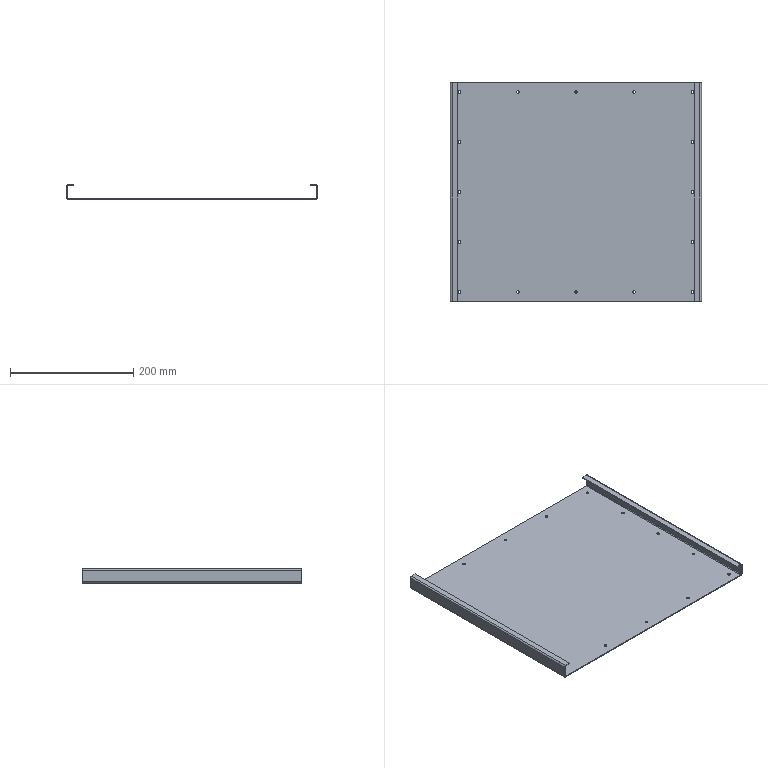Part | STEP file | Electrical box base plate | 1 solid | 54 faces | box 408 x 355 x 23 mm | volume 248875 mm3 | plane 30 | cylinder 24 | commonest cylinder face diameters 4.2 x16 2 x4 5 x4
STEP:
#1=CARTESIAN_POINT('',(10.,355.,-1.));
#2=VERTEX_POINT('',#1);
#3=CARTESIAN_POINT('',(11.5,355.,-1.));
#4=VERTEX_POINT('',#3);
#5=CARTESIAN_POINT('',(10.,355.,-1.));
#6=DIRECTION('',(1.,0.,0.));
#7=VECTOR('',#6,1000.);
#8=LINE('',#5,#7);
#9=EDGE_CURVE('',#2,#4,#8,.T.);
#10=ORIENTED_EDGE('',*,*,#9,.F.);
#11=CARTESIAN_POINT('',(9.,355.,0.));
#12=VERTEX_POINT('',#11);
#13=CARTESIAN_POINT('',(9.,355.,-1.));
#14=DIRECTION('',(0.,1.,0.));
#15=DIRECTION('',(0.,0.,-1.));
#16=AXIS2_PLACEMENT_3D('',#13,#14,#15);
#17=CIRCLE('',#16,1.);
#18=EDGE_CURVE('',#12,#2,#17,.T.);
#19=ORIENTED_EDGE('',*,*,#18,.F.);
#20=CARTESIAN_POINT('',(9.,355.,1.5));
#21=VERTEX_POINT('',#20);
#22=CARTESIAN_POINT('',(9.,355.,1.5));
#23=DIRECTION('',(0.,0.,-1.));
#24=VECTOR('',#23,1000.);
#25=LINE('',#22,#24);
#26=EDGE_CURVE('',#21,#12,#25,.T.);
#27=ORIENTED_EDGE('',*,*,#26,.F.);
#28=CARTESIAN_POINT('',(9.,355.,-1.));
#29=DIRECTION('',(0.,1.,0.));
#30=DIRECTION('',(1.,0.,0.));
#31=AXIS2_PLACEMENT_3D('',#28,#29,#30);
#32=CIRCLE('',#31,2.5);
#33=EDGE_CURVE('',#21,#4,#32,.T.);
#34=ORIENTED_EDGE('',*,*,#33,.T.);
#35=EDGE_LOOP('',(#10,#19,#27,#34));
#36=FACE_OUTER_BOUND('',#35,.T.);
#37=CARTESIAN_POINT('',(10.,355.,-1.));
#38=DIRECTION('',(0.,1.,0.));
#39=DIRECTION('',(0.,0.,1.));
#40=AXIS2_PLACEMENT_3D('',#37,#38,#39);
#41=PLANE('',#40);
#42=ADVANCED_FACE('',(#36),#41,.T.);
#43=CARTESIAN_POINT('',(10.,355.,-19.));
#44=VERTEX_POINT('',#43);
#45=CARTESIAN_POINT('',(10.,355.,0.));
#46=DIRECTION('',(0.,0.,-1.));
#47=VECTOR('',#46,1000.);
#48=LINE('',#45,#47);
#49=EDGE_CURVE('',#2,#44,#48,.T.);
#50=ORIENTED_EDGE('',*,*,#49,.F.);
#51=ORIENTED_EDGE('',*,*,#9,.T.);
#52=CARTESIAN_POINT('',(11.5,355.,-19.));
#53=VERTEX_POINT('',#52);
#54=CARTESIAN_POINT('',(11.5,355.,0.));
#55=DIRECTION('',(0.,0.,-1.));
#56=VECTOR('',#55,1000.);
#57=LINE('',#54,#56);
#58=EDGE_CURVE('',#4,#53,#57,.T.);
#59=ORIENTED_EDGE('',*,*,#58,.T.);
#60=CARTESIAN_POINT('',(11.5,355.,-19.));
#61=DIRECTION('',(-1.,0.,0.));
#62=VECTOR('',#61,1000.);
#63=LINE('',#60,#62);
#64=EDGE_CURVE('',#53,#44,#63,.T.);
#65=ORIENTED_EDGE('',*,*,#64,.T.);
#66=EDGE_LOOP('',(#50,#51,#59,#65));
#67=FACE_OUTER_BOUND('',#66,.T.);
#68=CARTESIAN_POINT('',(9.,355.,1.5));
#69=DIRECTION('',(0.,1.,0.));
#70=DIRECTION('',(0.,0.,1.));
#71=AXIS2_PLACEMENT_3D('',#68,#69,#70);
#72=PLANE('',#71);
#73=ADVANCED_FACE('',(#67),#72,.T.);
#74=CARTESIAN_POINT('',(9.,0.,0.));
#75=VERTEX_POINT('',#74);
#76=CARTESIAN_POINT('',(9.,0.,1.5));
#77=VERTEX_POINT('',#76);
#78=CARTESIAN_POINT('',(9.,0.,0.));
#79=DIRECTION('',(0.,0.,1.));
#80=VECTOR('',#79,1000.);
#81=LINE('',#78,#80);
#82=EDGE_CURVE('',#75,#77,#81,.T.);
#83=ORIENTED_EDGE('',*,*,#82,.F.);
#84=CARTESIAN_POINT('',(10.,0.,-1.));
#85=VERTEX_POINT('',#84);
#86=CARTESIAN_POINT('',(9.,0.,-1.));
#87=DIRECTION('',(0.,1.,0.));
#88=DIRECTION('',(0.,0.,-1.));
#89=AXIS2_PLACEMENT_3D('',#86,#87,#88);
#90=CIRCLE('',#89,1.);
#91=EDGE_CURVE('',#75,#85,#90,.T.);
#92=ORIENTED_EDGE('',*,*,#91,.T.);
#93=CARTESIAN_POINT('',(11.5,0.,-1.));
#94=VERTEX_POINT('',#93);
#95=CARTESIAN_POINT('',(11.5,0.,-1.));
#96=DIRECTION('',(-1.,0.,0.));
#97=VECTOR('',#96,1000.);
#98=LINE('',#95,#97);
#99=EDGE_CURVE('',#94,#85,#98,.T.);
#100=ORIENTED_EDGE('',*,*,#99,.F.);
#101=CARTESIAN_POINT('',(9.,0.,-1.));
#102=DIRECTION('',(0.,1.,0.));
#103=DIRECTION('',(1.,0.,0.));
#104=AXIS2_PLACEMENT_3D('',#101,#102,#103);
#105=CIRCLE('',#104,2.5);
#106=EDGE_CURVE('',#77,#94,#105,.T.);
#107=ORIENTED_EDGE('',*,*,#106,.F.);
#108=EDGE_LOOP('',(#83,#92,#100,#107));
#109=FACE_OUTER_BOUND('',#108,.T.);
#110=CARTESIAN_POINT('',(9.,0.,0.));
#111=DIRECTION('',(0.,-1.,0.));
#112=DIRECTION('',(0.,0.,-1.));
#113=AXIS2_PLACEMENT_3D('',#110,#111,#112);
#114=PLANE('',#113);
#115=ADVANCED_FACE('',(#109),#114,.T.);
#116=CARTESIAN_POINT('',(0.,0.,0.));
#117=VERTEX_POINT('',#116);
#118=CARTESIAN_POINT('',(0.,0.,0.));
#119=DIRECTION('',(1.,0.,0.));
#120=VECTOR('',#119,1000.);
#121=LINE('',#118,#120);
#122=EDGE_CURVE('',#117,#75,#121,.T.);
#123=ORIENTED_EDGE('',*,*,#122,.T.);
#124=ORIENTED_EDGE('',*,*,#82,.T.);
#125=CARTESIAN_POINT('',(0.,0.,1.5));
#126=VERTEX_POINT('',#125);
#127=CARTESIAN_POINT('',(0.,0.,1.5));
#128=DIRECTION('',(1.,0.,0.));
#129=VECTOR('',#128,1000.);
#130=LINE('',#127,#129);
#131=EDGE_CURVE('',#126,#77,#130,.T.);
#132=ORIENTED_EDGE('',*,*,#131,.F.);
#133=CARTESIAN_POINT('',(0.,0.,1.5));
#134=DIRECTION('',(0.,0.,-1.));
#135=VECTOR('',#134,1000.);
#136=LINE('',#133,#135);
#137=EDGE_CURVE('',#126,#117,#136,.T.);
#138=ORIENTED_EDGE('',*,*,#137,.T.);
#139=EDGE_LOOP('',(#123,#124,#132,#138));
#140=FACE_OUTER_BOUND('',#139,.T.);
#141=CARTESIAN_POINT('',(11.5,0.,-1.));
#142=DIRECTION('',(0.,-1.,0.));
#143=DIRECTION('',(0.,0.,-1.));
#144=AXIS2_PLACEMENT_3D('',#141,#142,#143);
#145=PLANE('',#144);
#146=ADVANCED_FACE('',(#140),#145,.T.);
#147=CARTESIAN_POINT('',(9.,355.,-20.));
#148=VERTEX_POINT('',#147);
#149=CARTESIAN_POINT('',(9.,355.,-21.5));
#150=VERTEX_POINT('',#149);
#151=CARTESIAN_POINT('',(9.,355.,-20.));
#152=DIRECTION('',(0.,0.,-1.));
#153=VECTOR('',#152,1000.);
#154=LINE('',#151,#153);
#155=EDGE_CURVE('',#148,#150,#154,.T.);
#156=ORIENTED_EDGE('',*,*,#155,.F.);
#157=CARTESIAN_POINT('',(9.,355.,-19.));
#158=DIRECTION('',(0.,1.,0.));
#159=DIRECTION('',(0.,0.,-1.));
#160=AXIS2_PLACEMENT_3D('',#157,#158,#159);
#161=CIRCLE('',#160,1.);
#162=EDGE_CURVE('',#44,#148,#161,.T.);
#163=ORIENTED_EDGE('',*,*,#162,.F.);
#164=ORIENTED_EDGE('',*,*,#64,.F.);
#165=CARTESIAN_POINT('',(9.,355.,-19.));
#166=DIRECTION('',(0.,1.,0.));
#167=DIRECTION('',(1.,0.,0.));
#168=AXIS2_PLACEMENT_3D('',#165,#166,#167);
#169=CIRCLE('',#168,2.5);
#170=EDGE_CURVE('',#53,#150,#169,.T.);
#171=ORIENTED_EDGE('',*,*,#170,.T.);
#172=EDGE_LOOP('',(#156,#163,#164,#171));
#173=FACE_OUTER_BOUND('',#172,.T.);
#174=CARTESIAN_POINT('',(9.,355.,-20.));
#175=DIRECTION('',(0.,1.,0.));
#176=DIRECTION('',(0.,0.,1.));
#177=AXIS2_PLACEMENT_3D('',#174,#175,#176);
#178=PLANE('',#177);
#179=ADVANCED_FACE('',(#173),#178,.T.);
#180=CARTESIAN_POINT('',(-394.,355.,-20.));
#181=VERTEX_POINT('',#180);
#182=CARTESIAN_POINT('',(10.,355.,-20.));
#183=DIRECTION('',(-1.,0.,0.));
#184=VECTOR('',#183,1000.);
#185=LINE('',#182,#184);
#186=EDGE_CURVE('',#148,#181,#185,.T.);
#187=ORIENTED_EDGE('',*,*,#186,.F.);
#188=ORIENTED_EDGE('',*,*,#155,.T.);
#189=CARTESIAN_POINT('',(-394.,355.,-21.5));
#190=VERTEX_POINT('',#189);
#191=CARTESIAN_POINT('',(10.,355.,-21.5));
#192=DIRECTION('',(-1.,0.,0.));
#193=VECTOR('',#192,1000.);
#194=LINE('',#191,#193);
#195=EDGE_CURVE('',#150,#190,#194,.T.);
#196=ORIENTED_EDGE('',*,*,#195,.T.);
#197=CARTESIAN_POINT('',(-394.,355.,-21.5));
#198=DIRECTION('',(0.,0.,1.));
#199=VECTOR('',#198,1000.);
#200=LINE('',#197,#199);
#201=EDGE_CURVE('',#190,#181,#200,.T.);
#202=ORIENTED_EDGE('',*,*,#201,.T.);
#203=EDGE_LOOP('',(#187,#188,#196,#202));
#204=FACE_OUTER_BOUND('',#203,.T.);
#205=CARTESIAN_POINT('',(11.5,355.,-19.));
#206=DIRECTION('',(0.,1.,0.));
#207=DIRECTION('',(0.,0.,1.));
#208=AXIS2_PLACEMENT_3D('',#205,#206,#207);
#209=PLANE('',#208);
#210=ADVANCED_FACE('',(#204),#209,.T.);
#211=CARTESIAN_POINT('',(10.,0.,-19.));
#212=VERTEX_POINT('',#211);
#213=CARTESIAN_POINT('',(11.5,0.,-19.));
#214=VERTEX_POINT('',#213);
#215=CARTESIAN_POINT('',(10.,0.,-19.));
#216=DIRECTION('',(1.,0.,0.));
#217=VECTOR('',#216,1000.);
#218=LINE('',#215,#217);
#219=EDGE_CURVE('',#212,#214,#218,.T.);
#220=ORIENTED_EDGE('',*,*,#219,.F.);
#221=CARTESIAN_POINT('',(9.,0.,-20.));
#222=VERTEX_POINT('',#221);
#223=CARTESIAN_POINT('',(9.,0.,-19.));
#224=DIRECTION('',(0.,1.,0.));
#225=DIRECTION('',(0.,0.,-1.));
#226=AXIS2_PLACEMENT_3D('',#223,#224,#225);
#227=CIRCLE('',#226,1.);
#228=EDGE_CURVE('',#212,#222,#227,.T.);
#229=ORIENTED_EDGE('',*,*,#228,.T.);
#230=CARTESIAN_POINT('',(9.,0.,-21.5));
#231=VERTEX_POINT('',#230);
#232=CARTESIAN_POINT('',(9.,0.,-21.5));
#233=DIRECTION('',(0.,0.,1.));
#234=VECTOR('',#233,1000.);
#235=LINE('',#232,#234);
#236=EDGE_CURVE('',#231,#222,#235,.T.);
#237=ORIENTED_EDGE('',*,*,#236,.F.);
#238=CARTESIAN_POINT('',(9.,0.,-19.));
#239=DIRECTION('',(0.,1.,0.));
#240=DIRECTION('',(1.,0.,0.));
#241=AXIS2_PLACEMENT_3D('',#238,#239,#240);
#242=CIRCLE('',#241,2.5);
#243=EDGE_CURVE('',#214,#231,#242,.T.);
#244=ORIENTED_EDGE('',*,*,#243,.F.);
#245=EDGE_LOOP('',(#220,#229,#237,#244));
#246=FACE_OUTER_BOUND('',#245,.T.);
#247=CARTESIAN_POINT('',(10.,0.,-19.));
#248=DIRECTION('',(0.,-1.,0.));
#249=DIRECTION('',(0.,0.,-1.));
#250=AXIS2_PLACEMENT_3D('',#247,#248,#249);
#251=PLANE('',#250);
#252=ADVANCED_FACE('',(#246),#251,.T.);
#253=CARTESIAN_POINT('',(10.,0.,0.));
#254=DIRECTION('',(0.,0.,-1.));
#255=VECTOR('',#254,1000.);
#256=LINE('',#253,#255);
#257=EDGE_CURVE('',#85,#212,#256,.T.);
#258=ORIENTED_EDGE('',*,*,#257,.T.);
#259=ORIENTED_EDGE('',*,*,#219,.T.);
#260=CARTESIAN_POINT('',(11.5,0.,0.));
#261=DIRECTION('',(0.,0.,-1.));
#262=VECTOR('',#261,1000.);
#263=LINE('',#260,#262);
#264=EDGE_CURVE('',#94,#214,#263,.T.);
#265=ORIENTED_EDGE('',*,*,#264,.F.);
#266=ORIENTED_EDGE('',*,*,#99,.T.);
#267=EDGE_LOOP('',(#258,#259,#265,#266));
#268=FACE_OUTER_BOUND('',#267,.T.);
#269=CARTESIAN_POINT('',(9.,0.,-21.5));
#270=DIRECTION('',(0.,-1.,0.));
#271=DIRECTION('',(0.,0.,-1.));
#272=AXIS2_PLACEMENT_3D('',#269,#270,#271);
#273=PLANE('',#272);
#274=ADVANCED_FACE('',(#268),#273,.T.);
#275=CARTESIAN_POINT('',(-395.,355.,-19.));
#276=VERTEX_POINT('',#275);
#277=CARTESIAN_POINT('',(-396.5,355.,-19.));
#278=VERTEX_POINT('',#277);
#279=CARTESIAN_POINT('',(-395.,355.,-19.));
#280=DIRECTION('',(-1.,0.,0.));
#281=VECTOR('',#280,1000.);
#282=LINE('',#279,#281);
#283=EDGE_CURVE('',#276,#278,#282,.T.);
#284=ORIENTED_EDGE('',*,*,#283,.F.);
#285=CARTESIAN_POINT('',(-394.,355.,-19.));
#286=DIRECTION('',(0.,1.,0.));
#287=DIRECTION('',(0.,0.,-1.));
#288=AXIS2_PLACEMENT_3D('',#285,#286,#287);
#289=CIRCLE('',#288,1.);
#290=EDGE_CURVE('',#181,#276,#289,.T.);
#291=ORIENTED_EDGE('',*,*,#290,.F.);
#292=ORIENTED_EDGE('',*,*,#201,.F.);
#293=CARTESIAN_POINT('',(-394.,355.,-19.));
#294=DIRECTION('',(0.,1.,0.));
#295=DIRECTION('',(1.,0.,0.));
#296=AXIS2_PLACEMENT_3D('',#293,#294,#295);
#297=CIRCLE('',#296,2.5);
#298=EDGE_CURVE('',#190,#278,#297,.T.);
#299=ORIENTED_EDGE('',*,*,#298,.T.);
#300=EDGE_LOOP('',(#284,#291,#292,#299));
#301=FACE_OUTER_BOUND('',#300,.T.);
#302=CARTESIAN_POINT('',(-395.,355.,-19.));
#303=DIRECTION('',(0.,1.,0.));
#304=DIRECTION('',(0.,0.,1.));
#305=AXIS2_PLACEMENT_3D('',#302,#303,#304);
#306=PLANE('',#305);
#307=ADVANCED_FACE('',(#301),#306,.T.);
#308=CARTESIAN_POINT('',(-395.,355.,-1.));
#309=VERTEX_POINT('',#308);
#310=CARTESIAN_POINT('',(-395.,355.,-20.));
#311=DIRECTION('',(0.,0.,1.));
#312=VECTOR('',#311,1000.);
#313=LINE('',#310,#312);
#314=EDGE_CURVE('',#276,#309,#313,.T.);
#315=ORIENTED_EDGE('',*,*,#314,.F.);
#316=ORIENTED_EDGE('',*,*,#283,.T.);
#317=CARTESIAN_POINT('',(-396.5,355.,-1.));
#318=VERTEX_POINT('',#317);
#319=CARTESIAN_POINT('',(-396.5,355.,-20.));
#320=DIRECTION('',(0.,0.,1.));
#321=VECTOR('',#320,1000.);
#322=LINE('',#319,#321);
#323=EDGE_CURVE('',#278,#318,#322,.T.);
#324=ORIENTED_EDGE('',*,*,#323,.T.);
#325=CARTESIAN_POINT('',(-396.5,355.,-1.));
#326=DIRECTION('',(1.,0.,0.));
#327=VECTOR('',#326,1000.);
#328=LINE('',#325,#327);
#329=EDGE_CURVE('',#318,#309,#328,.T.);
#330=ORIENTED_EDGE('',*,*,#329,.T.);
#331=EDGE_LOOP('',(#315,#316,#324,#330));
#332=FACE_OUTER_BOUND('',#331,.T.);
#333=CARTESIAN_POINT('',(-394.,355.,-21.5));
#334=DIRECTION('',(0.,1.,0.));
#335=DIRECTION('',(0.,0.,1.));
#336=AXIS2_PLACEMENT_3D('',#333,#334,#335);
#337=PLANE('',#336);
#338=ADVANCED_FACE('',(#332),#337,.T.);
#339=CARTESIAN_POINT('',(-394.,0.,-20.));
#340=VERTEX_POINT('',#339);
#341=CARTESIAN_POINT('',(-394.,0.,-21.5));
#342=VERTEX_POINT('',#341);
#343=CARTESIAN_POINT('',(-394.,0.,-20.));
#344=DIRECTION('',(0.,0.,-1.));
#345=VECTOR('',#344,1000.);
#346=LINE('',#343,#345);
#347=EDGE_CURVE('',#340,#342,#346,.T.);
#348=ORIENTED_EDGE('',*,*,#347,.F.);
#349=CARTESIAN_POINT('',(-395.,0.,-19.));
#350=VERTEX_POINT('',#349);
#351=CARTESIAN_POINT('',(-394.,0.,-19.));
#352=DIRECTION('',(0.,1.,0.));
#353=DIRECTION('',(0.,0.,-1.));
#354=AXIS2_PLACEMENT_3D('',#351,#352,#353);
#355=CIRCLE('',#354,1.);
#356=EDGE_CURVE('',#340,#350,#355,.T.);
#357=ORIENTED_EDGE('',*,*,#356,.T.);
#358=CARTESIAN_POINT('',(-396.5,0.,-19.));
#359=VERTEX_POINT('',#358);
#360=CARTESIAN_POINT('',(-396.5,0.,-19.));
#361=DIRECTION('',(1.,0.,0.));
#362=VECTOR('',#361,1000.);
#363=LINE('',#360,#362);
#364=EDGE_CURVE('',#359,#350,#363,.T.);
#365=ORIENTED_EDGE('',*,*,#364,.F.);
#366=CARTESIAN_POINT('',(-394.,0.,-19.));
#367=DIRECTION('',(0.,1.,0.));
#368=DIRECTION('',(1.,0.,0.));
#369=AXIS2_PLACEMENT_3D('',#366,#367,#368);
#370=CIRCLE('',#369,2.5);
#371=EDGE_CURVE('',#342,#359,#370,.T.);
#372=ORIENTED_EDGE('',*,*,#371,.F.);
#373=EDGE_LOOP('',(#348,#357,#365,#372));
#374=FACE_OUTER_BOUND('',#373,.T.);
#375=CARTESIAN_POINT('',(-394.,0.,-20.));
#376=DIRECTION('',(0.,-1.,0.));
#377=DIRECTION('',(0.,0.,-1.));
#378=AXIS2_PLACEMENT_3D('',#375,#376,#377);
#379=PLANE('',#378);
#380=ADVANCED_FACE('',(#374),#379,.T.);
#381=CARTESIAN_POINT('',(10.,0.,-20.));
#382=DIRECTION('',(-1.,0.,0.));
#383=VECTOR('',#382,1000.);
#384=LINE('',#381,#383);
#385=EDGE_CURVE('',#222,#340,#384,.T.);
#386=ORIENTED_EDGE('',*,*,#385,.T.);
#387=ORIENTED_EDGE('',*,*,#347,.T.);
#388=CARTESIAN_POINT('',(10.,0.,-21.5));
#389=DIRECTION('',(-1.,0.,0.));
#390=VECTOR('',#389,1000.);
#391=LINE('',#388,#390);
#392=EDGE_CURVE('',#231,#342,#391,.T.);
#393=ORIENTED_EDGE('',*,*,#392,.F.);
#394=ORIENTED_EDGE('',*,*,#236,.T.);
#395=EDGE_LOOP('',(#386,#387,#393,#394));
#396=FACE_OUTER_BOUND('',#395,.T.);
#397=CARTESIAN_POINT('',(-396.5,0.,-19.));
#398=DIRECTION('',(0.,-1.,0.));
#399=DIRECTION('',(0.,0.,-1.));
#400=AXIS2_PLACEMENT_3D('',#397,#398,#399);
#401=PLANE('',#400);
#402=ADVANCED_FACE('',(#396),#401,.T.);
#403=CARTESIAN_POINT('',(-394.,355.,0.));
#404=VERTEX_POINT('',#403);
#405=CARTESIAN_POINT('',(-394.,355.,1.5));
#406=VERTEX_POINT('',#405);
#407=CARTESIAN_POINT('',(-394.,355.,0.));
#408=DIRECTION('',(0.,0.,1.));
#409=VECTOR('',#408,1000.);
#410=LINE('',#407,#409);
#411=EDGE_CURVE('',#404,#406,#410,.T.);
#412=ORIENTED_EDGE('',*,*,#411,.F.);
#413=CARTESIAN_POINT('',(-394.,355.,-1.));
#414=DIRECTION('',(0.,1.,0.));
#415=DIRECTION('',(0.,0.,-1.));
#416=AXIS2_PLACEMENT_3D('',#413,#414,#415);
#417=CIRCLE('',#416,1.);
#418=EDGE_CURVE('',#309,#404,#417,.T.);
#419=ORIENTED_EDGE('',*,*,#418,.F.);
#420=ORIENTED_EDGE('',*,*,#329,.F.);
#421=CARTESIAN_POINT('',(-394.,355.,-1.));
#422=DIRECTION('',(0.,1.,0.));
#423=DIRECTION('',(1.,0.,0.));
#424=AXIS2_PLACEMENT_3D('',#421,#422,#423);
#425=CIRCLE('',#424,2.5);
#426=EDGE_CURVE('',#318,#406,#425,.T.);
#427=ORIENTED_EDGE('',*,*,#426,.T.);
#428=EDGE_LOOP('',(#412,#419,#420,#427));
#429=FACE_OUTER_BOUND('',#428,.T.);
#430=CARTESIAN_POINT('',(-394.,355.,0.));
#431=DIRECTION('',(0.,1.,0.));
#432=DIRECTION('',(0.,0.,1.));
#433=AXIS2_PLACEMENT_3D('',#430,#431,#432);
#434=PLANE('',#433);
#435=ADVANCED_FACE('',(#429),#434,.T.);
#436=CARTESIAN_POINT('',(-385.,355.,0.));
#437=VERTEX_POINT('',#436);
#438=CARTESIAN_POINT('',(-395.,355.,0.));
#439=DIRECTION('',(1.,0.,0.));
#440=VECTOR('',#439,1000.);
#441=LINE('',#438,#440);
#442=EDGE_CURVE('',#404,#437,#441,.T.);
#443=ORIENTED_EDGE('',*,*,#442,.F.);
#444=ORIENTED_EDGE('',*,*,#411,.T.);
#445=CARTESIAN_POINT('',(-385.,355.,1.5));
#446=VERTEX_POINT('',#445);
#447=CARTESIAN_POINT('',(-395.,355.,1.5));
#448=DIRECTION('',(1.,0.,0.));
#449=VECTOR('',#448,1000.);
#450=LINE('',#447,#449);
#451=EDGE_CURVE('',#406,#446,#450,.T.);
#452=ORIENTED_EDGE('',*,*,#451,.T.);
#453=CARTESIAN_POINT('',(-385.,355.,0.));
#454=DIRECTION('',(0.,0.,1.));
#455=VECTOR('',#454,1000.);
#456=LINE('',#453,#455);
#457=EDGE_CURVE('',#437,#446,#456,.T.);
#458=ORIENTED_EDGE('',*,*,#457,.F.);
#459=EDGE_LOOP('',(#443,#444,#452,#458));
#460=FACE_OUTER_BOUND('',#459,.T.);
#461=CARTESIAN_POINT('',(-396.5,355.,-1.));
#462=DIRECTION('',(0.,1.,0.));
#463=DIRECTION('',(0.,0.,1.));
#464=AXIS2_PLACEMENT_3D('',#461,#462,#463);
#465=PLANE('',#464);
#466=ADVANCED_FACE('',(#460),#465,.T.);
#467=CARTESIAN_POINT('',(-395.,0.,-1.));
#468=VERTEX_POINT('',#467);
#469=CARTESIAN_POINT('',(-396.5,0.,-1.));
#470=VERTEX_POINT('',#469);
#471=CARTESIAN_POINT('',(-395.,0.,-1.));
#472=DIRECTION('',(-1.,0.,0.));
#473=VECTOR('',#472,1000.);
#474=LINE('',#471,#473);
#475=EDGE_CURVE('',#468,#470,#474,.T.);
#476=ORIENTED_EDGE('',*,*,#475,.F.);
#477=CARTESIAN_POINT('',(-394.,0.,0.));
#478=VERTEX_POINT('',#477);
#479=CARTESIAN_POINT('',(-394.,0.,-1.));
#480=DIRECTION('',(0.,1.,0.));
#481=DIRECTION('',(0.,0.,-1.));
#482=AXIS2_PLACEMENT_3D('',#479,#480,#481);
#483=CIRCLE('',#482,1.);
#484=EDGE_CURVE('',#468,#478,#483,.T.);
#485=ORIENTED_EDGE('',*,*,#484,.T.);
#486=CARTESIAN_POINT('',(-394.,0.,1.5));
#487=VERTEX_POINT('',#486);
#488=CARTESIAN_POINT('',(-394.,0.,1.5));
#489=DIRECTION('',(0.,0.,-1.));
#490=VECTOR('',#489,1000.);
#491=LINE('',#488,#490);
#492=EDGE_CURVE('',#487,#478,#491,.T.);
#493=ORIENTED_EDGE('',*,*,#492,.F.);
#494=CARTESIAN_POINT('',(-394.,0.,-1.));
#495=DIRECTION('',(0.,1.,0.));
#496=DIRECTION('',(1.,0.,0.));
#497=AXIS2_PLACEMENT_3D('',#494,#495,#496);
#498=CIRCLE('',#497,2.5);
#499=EDGE_CURVE('',#470,#487,#498,.T.);
#500=ORIENTED_EDGE('',*,*,#499,.F.);
#501=EDGE_LOOP('',(#476,#485,#493,#500));
#502=FACE_OUTER_BOUND('',#501,.T.);
#503=CARTESIAN_POINT('',(-395.,0.,-1.));
#504=DIRECTION('',(0.,-1.,0.));
#505=DIRECTION('',(0.,0.,-1.));
#506=AXIS2_PLACEMENT_3D('',#503,#504,#505);
#507=PLANE('',#506);
#508=ADVANCED_FACE('',(#502),#507,.T.);
#509=CARTESIAN_POINT('',(-395.,0.,-20.));
#510=DIRECTION('',(0.,0.,1.));
#511=VECTOR('',#510,1000.);
#512=LINE('',#509,#511);
#513=EDGE_CURVE('',#350,#468,#512,.T.);
#514=ORIENTED_EDGE('',*,*,#513,.T.);
#515=ORIENTED_EDGE('',*,*,#475,.T.);
#516=CARTESIAN_POINT('',(-396.5,0.,-20.));
#517=DIRECTION('',(0.,0.,1.));
#518=VECTOR('',#517,1000.);
#519=LINE('',#516,#518);
#520=EDGE_CURVE('',#359,#470,#519,.T.);
#521=ORIENTED_EDGE('',*,*,#520,.F.);
#522=ORIENTED_EDGE('',*,*,#364,.T.);
#523=EDGE_LOOP('',(#514,#515,#521,#522));
#524=FACE_OUTER_BOUND('',#523,.T.);
#525=CARTESIAN_POINT('',(-394.,0.,1.5));
#526=DIRECTION('',(0.,-1.,0.));
#527=DIRECTION('',(0.,0.,-1.));
#528=AXIS2_PLACEMENT_3D('',#525,#526,#527);
#529=PLANE('',#528);
#530=ADVANCED_FACE('',(#524),#529,.T.);
#531=CARTESIAN_POINT('',(-385.,0.,1.5));
#532=VERTEX_POINT('',#531);
#533=CARTESIAN_POINT('',(-395.,0.,1.5));
#534=DIRECTION('',(1.,0.,0.));
#535=VECTOR('',#534,1000.);
#536=LINE('',#533,#535);
#537=EDGE_CURVE('',#487,#532,#536,.T.);
#538=ORIENTED_EDGE('',*,*,#537,.T.);
#539=CARTESIAN_POINT('',(-385.,355.,1.5));
#540=DIRECTION('',(0.,-1.,0.));
#541=VECTOR('',#540,1000.);
#542=LINE('',#539,#541);
#543=EDGE_CURVE('',#446,#532,#542,.T.);
#544=ORIENTED_EDGE('',*,*,#543,.F.);
#545=ORIENTED_EDGE('',*,*,#451,.F.);
#546=CARTESIAN_POINT('',(-394.,355.,1.5));
#547=DIRECTION('',(0.,-1.,0.));
#548=VECTOR('',#547,1000.);
#549=LINE('',#546,#548);
#550=EDGE_CURVE('',#406,#487,#549,.T.);
#551=ORIENTED_EDGE('',*,*,#550,.T.);
#552=EDGE_LOOP('',(#538,#544,#545,#551));
#553=FACE_OUTER_BOUND('',#552,.T.);
#554=CARTESIAN_POINT('',(-395.,355.,1.5));
#555=DIRECTION('',(0.,0.,-1.));
#556=DIRECTION('',(-1.,0.,0.));
#557=AXIS2_PLACEMENT_3D('',#554,#555,#556);
#558=PLANE('',#557);
#559=ADVANCED_FACE('',(#553),#558,.F.);
#560=CARTESIAN_POINT('',(-385.,0.,0.));
#561=VERTEX_POINT('',#560);
#562=CARTESIAN_POINT('',(-385.,0.,0.));
#563=DIRECTION('',(0.,0.,1.));
#564=VECTOR('',#563,1000.);
#565=LINE('',#562,#564);
#566=EDGE_CURVE('',#561,#532,#565,.T.);
#567=ORIENTED_EDGE('',*,*,#566,.F.);
#568=CARTESIAN_POINT('',(-385.,355.,0.));
#569=DIRECTION('',(0.,-1.,0.));
#570=VECTOR('',#569,1000.);
#571=LINE('',#568,#570);
#572=EDGE_CURVE('',#437,#561,#571,.T.);
#573=ORIENTED_EDGE('',*,*,#572,.F.);
#574=ORIENTED_EDGE('',*,*,#457,.T.);
#575=ORIENTED_EDGE('',*,*,#543,.T.);
#576=EDGE_LOOP('',(#567,#573,#574,#575));
#577=FACE_OUTER_BOUND('',#576,.T.);
#578=CARTESIAN_POINT('',(-385.,355.,0.));
#579=DIRECTION('',(1.,0.,0.));
#580=DIRECTION('',(0.,0.,-1.));
#581=AXIS2_PLACEMENT_3D('',#578,#579,#580);
#582=PLANE('',#581);
#583=ADVANCED_FACE('',(#577),#582,.T.);
#584=CARTESIAN_POINT('',(-395.,0.,0.));
#585=DIRECTION('',(1.,0.,0.));
#586=VECTOR('',#585,1000.);
#587=LINE('',#584,#586);
#588=EDGE_CURVE('',#478,#561,#587,.T.);
#589=ORIENTED_EDGE('',*,*,#588,.F.);
#590=CARTESIAN_POINT('',(-394.,355.,0.));
#591=DIRECTION('',(0.,-1.,0.));
#592=VECTOR('',#591,1000.);
#593=LINE('',#590,#592);
#594=EDGE_CURVE('',#404,#478,#593,.T.);
#595=ORIENTED_EDGE('',*,*,#594,.F.);
#596=ORIENTED_EDGE('',*,*,#442,.T.);
#597=ORIENTED_EDGE('',*,*,#572,.T.);
#598=EDGE_LOOP('',(#589,#595,#596,#597));
#599=FACE_OUTER_BOUND('',#598,.T.);
#600=CARTESIAN_POINT('',(-395.,355.,0.));
#601=DIRECTION('',(0.,0.,-1.));
#602=DIRECTION('',(-1.,0.,0.));
#603=AXIS2_PLACEMENT_3D('',#600,#601,#602);
#604=PLANE('',#603);
#605=ADVANCED_FACE('',(#599),#604,.T.);
#606=ORIENTED_EDGE('',*,*,#484,.F.);
#607=CARTESIAN_POINT('',(-395.,355.,-1.));
#608=DIRECTION('',(0.,-1.,0.));
#609=VECTOR('',#608,1000.);
#610=LINE('',#607,#609);
#611=EDGE_CURVE('',#309,#468,#610,.T.);
#612=ORIENTED_EDGE('',*,*,#611,.F.);
#613=ORIENTED_EDGE('',*,*,#418,.T.);
#614=ORIENTED_EDGE('',*,*,#594,.T.);
#615=EDGE_LOOP('',(#606,#612,#613,#614));
#616=FACE_OUTER_BOUND('',#615,.T.);
#617=CARTESIAN_POINT('',(-394.,355.,-1.));
#618=DIRECTION('',(0.,-1.,0.));
#619=DIRECTION('',(0.,0.,-1.));
#620=AXIS2_PLACEMENT_3D('',#617,#618,#619);
#621=CYLINDRICAL_SURFACE('',#620,1.);
#622=ADVANCED_FACE('',(#616),#621,.F.);
#623=ORIENTED_EDGE('',*,*,#513,.F.);
#624=CARTESIAN_POINT('',(-395.,355.,-19.));
#625=DIRECTION('',(0.,-1.,0.));
#626=VECTOR('',#625,1000.);
#627=LINE('',#624,#626);
#628=EDGE_CURVE('',#276,#350,#627,.T.);
#629=ORIENTED_EDGE('',*,*,#628,.F.);
#630=ORIENTED_EDGE('',*,*,#314,.T.);
#631=ORIENTED_EDGE('',*,*,#611,.T.);
#632=EDGE_LOOP('',(#623,#629,#630,#631));
#633=FACE_OUTER_BOUND('',#632,.T.);
#634=CARTESIAN_POINT('',(-395.,355.,-20.));
#635=DIRECTION('',(1.,0.,0.));
#636=DIRECTION('',(0.,0.,-1.));
#637=AXIS2_PLACEMENT_3D('',#634,#635,#636);
#638=PLANE('',#637);
#639=ADVANCED_FACE('',(#633),#638,.T.);
#640=ORIENTED_EDGE('',*,*,#356,.F.);
#641=CARTESIAN_POINT('',(-394.,355.,-20.));
#642=DIRECTION('',(0.,-1.,0.));
#643=VECTOR('',#642,1000.);
#644=LINE('',#641,#643);
#645=EDGE_CURVE('',#181,#340,#644,.T.);
#646=ORIENTED_EDGE('',*,*,#645,.F.);
#647=ORIENTED_EDGE('',*,*,#290,.T.);
#648=ORIENTED_EDGE('',*,*,#628,.T.);
#649=EDGE_LOOP('',(#640,#646,#647,#648));
#650=FACE_OUTER_BOUND('',#649,.T.);
#651=CARTESIAN_POINT('',(-394.,355.,-19.));
#652=DIRECTION('',(0.,-1.,0.));
#653=DIRECTION('',(0.,0.,-1.));
#654=AXIS2_PLACEMENT_3D('',#651,#652,#653);
#655=CYLINDRICAL_SURFACE('',#654,1.);
#656=ADVANCED_FACE('',(#650),#655,.F.);
#657=CARTESIAN_POINT('',(-379.4,15.,-20.));
#658=VERTEX_POINT('',#657);
#659=CARTESIAN_POINT('',(-381.5,15.,-20.));
#660=DIRECTION('',(0.,0.,1.));
#661=DIRECTION('',(1.,0.,0.));
#662=AXIS2_PLACEMENT_3D('',#659,#660,#661);
#663=CIRCLE('',#662,2.1);
#664=EDGE_CURVE('',#658,#658,#663,.T.);
#665=ORIENTED_EDGE('',*,*,#664,.F.);
#666=EDGE_LOOP('',(#665));
#667=FACE_BOUND('',#666,.T.);
#668=CARTESIAN_POINT('',(-284.9,15.,-20.));
#669=VERTEX_POINT('',#668);
#670=CARTESIAN_POINT('',(-287.,15.,-20.));
#671=DIRECTION('',(0.,0.,1.));
#672=DIRECTION('',(1.,0.,0.));
#673=AXIS2_PLACEMENT_3D('',#670,#671,#672);
#674=CIRCLE('',#673,2.1);
#675=EDGE_CURVE('',#669,#669,#674,.T.);
#676=ORIENTED_EDGE('',*,*,#675,.F.);
#677=EDGE_LOOP('',(#676));
#678=FACE_BOUND('',#677,.T.);
#679=CARTESIAN_POINT('',(-190.4,15.,-20.));
#680=VERTEX_POINT('',#679);
#681=CARTESIAN_POINT('',(-192.5,15.,-20.));
#682=DIRECTION('',(0.,0.,1.));
#683=DIRECTION('',(1.,0.,0.));
#684=AXIS2_PLACEMENT_3D('',#681,#682,#683);
#685=CIRCLE('',#684,2.1);
#686=EDGE_CURVE('',#680,#680,#685,.T.);
#687=ORIENTED_EDGE('',*,*,#686,.F.);
#688=EDGE_LOOP('',(#687));
#689=FACE_BOUND('',#688,.T.);
#690=CARTESIAN_POINT('',(-95.9,15.,-20.));
#691=VERTEX_POINT('',#690);
#692=CARTESIAN_POINT('',(-98.,15.,-20.));
#693=DIRECTION('',(0.,0.,1.));
#694=DIRECTION('',(1.,0.,0.));
#695=AXIS2_PLACEMENT_3D('',#692,#693,#694);
#696=CIRCLE('',#695,2.1);
#697=EDGE_CURVE('',#691,#691,#696,.T.);
#698=ORIENTED_EDGE('',*,*,#697,.F.);
#699=EDGE_LOOP('',(#698));
#700=FACE_BOUND('',#699,.T.);
#701=CARTESIAN_POINT('',(-1.4,15.,-20.));
#702=VERTEX_POINT('',#701);
#703=CARTESIAN_POINT('',(-3.5,15.,-20.));
#704=DIRECTION('',(0.,0.,1.));
#705=DIRECTION('',(1.,0.,0.));
#706=AXIS2_PLACEMENT_3D('',#703,#704,#705);
#707=CIRCLE('',#706,2.1);
#708=EDGE_CURVE('',#702,#702,#707,.T.);
#709=ORIENTED_EDGE('',*,*,#708,.F.);
#710=EDGE_LOOP('',(#709));
#711=FACE_BOUND('',#710,.T.);
#712=CARTESIAN_POINT('',(-1.4,340.,-20.));
#713=VERTEX_POINT('',#712);
#714=CARTESIAN_POINT('',(-3.5,340.,-20.));
#715=DIRECTION('',(0.,0.,1.));
#716=DIRECTION('',(1.,0.,0.));
#717=AXIS2_PLACEMENT_3D('',#714,#715,#716);
#718=CIRCLE('',#717,2.1);
#719=EDGE_CURVE('',#713,#713,#718,.T.);
#720=ORIENTED_EDGE('',*,*,#719,.F.);
#721=EDGE_LOOP('',(#720));
#722=FACE_BOUND('',#721,.T.);
#723=CARTESIAN_POINT('',(-95.9,340.,-20.));
#724=VERTEX_POINT('',#723);
#725=CARTESIAN_POINT('',(-98.,340.,-20.));
#726=DIRECTION('',(0.,0.,1.));
#727=DIRECTION('',(1.,0.,0.));
#728=AXIS2_PLACEMENT_3D('',#725,#726,#727);
#729=CIRCLE('',#728,2.1);
#730=EDGE_CURVE('',#724,#724,#729,.T.);
#731=ORIENTED_EDGE('',*,*,#730,.F.);
#732=EDGE_LOOP('',(#731));
#733=FACE_BOUND('',#732,.T.);
#734=CARTESIAN_POINT('',(-190.4,340.,-20.));
#735=VERTEX_POINT('',#734);
#736=CARTESIAN_POINT('',(-192.5,340.,-20.));
#737=DIRECTION('',(0.,0.,1.));
#738=DIRECTION('',(1.,0.,0.));
#739=AXIS2_PLACEMENT_3D('',#736,#737,#738);
#740=CIRCLE('',#739,2.1);
#741=EDGE_CURVE('',#735,#735,#740,.T.);
#742=ORIENTED_EDGE('',*,*,#741,.F.);
#743=EDGE_LOOP('',(#742));
#744=FACE_BOUND('',#743,.T.);
#745=CARTESIAN_POINT('',(-284.9,340.,-20.));
#746=VERTEX_POINT('',#745);
#747=CARTESIAN_POINT('',(-287.,340.,-20.));
#748=DIRECTION('',(0.,0.,1.));
#749=DIRECTION('',(1.,0.,0.));
#750=AXIS2_PLACEMENT_3D('',#747,#748,#749);
#751=CIRCLE('',#750,2.1);
#752=EDGE_CURVE('',#746,#746,#751,.T.);
#753=ORIENTED_EDGE('',*,*,#752,.F.);
#754=EDGE_LOOP('',(#753));
#755=FACE_BOUND('',#754,.T.);
#756=CARTESIAN_POINT('',(-379.4,96.25,-20.));
#757=VERTEX_POINT('',#756);
#758=CARTESIAN_POINT('',(-381.5,96.25,-20.));
#759=DIRECTION('',(0.,0.,1.));
#760=DIRECTION('',(1.,0.,0.));
#761=AXIS2_PLACEMENT_3D('',#758,#759,#760);
#762=CIRCLE('',#761,2.1);
#763=EDGE_CURVE('',#757,#757,#762,.T.);
#764=ORIENTED_EDGE('',*,*,#763,.F.);
#765=EDGE_LOOP('',(#764));
#766=FACE_BOUND('',#765,.T.);
#767=CARTESIAN_POINT('',(-379.4,177.5,-20.));
#768=VERTEX_POINT('',#767);
#769=CARTESIAN_POINT('',(-381.5,177.5,-20.));
#770=DIRECTION('',(0.,0.,1.));
#771=DIRECTION('',(1.,0.,0.));
#772=AXIS2_PLACEMENT_3D('',#769,#770,#771);
#773=CIRCLE('',#772,2.1);
#774=EDGE_CURVE('',#768,#768,#773,.T.);
#775=ORIENTED_EDGE('',*,*,#774,.F.);
#776=EDGE_LOOP('',(#775));
#777=FACE_BOUND('',#776,.T.);
#778=CARTESIAN_POINT('',(-379.4,258.75,-20.));
#779=VERTEX_POINT('',#778);
#780=CARTESIAN_POINT('',(-381.5,258.75,-20.));
#781=DIRECTION('',(0.,0.,1.));
#782=DIRECTION('',(1.,0.,0.));
#783=AXIS2_PLACEMENT_3D('',#780,#781,#782);
#784=CIRCLE('',#783,2.1);
#785=EDGE_CURVE('',#779,#779,#784,.T.);
#786=ORIENTED_EDGE('',*,*,#785,.F.);
#787=EDGE_LOOP('',(#786));
#788=FACE_BOUND('',#787,.T.);
#789=CARTESIAN_POINT('',(-379.4,340.,-20.));
#790=VERTEX_POINT('',#789);
#791=CARTESIAN_POINT('',(-381.5,340.,-20.));
#792=DIRECTION('',(0.,0.,1.));
#793=DIRECTION('',(1.,0.,0.));
#794=AXIS2_PLACEMENT_3D('',#791,#792,#793);
#795=CIRCLE('',#794,2.1);
#796=EDGE_CURVE('',#790,#790,#795,.T.);
#797=ORIENTED_EDGE('',*,*,#796,.F.);
#798=EDGE_LOOP('',(#797));
#799=FACE_BOUND('',#798,.T.);
#800=CARTESIAN_POINT('',(-1.4,258.75,-20.));
#801=VERTEX_POINT('',#800);
#802=CARTESIAN_POINT('',(-3.5,258.75,-20.));
#803=DIRECTION('',(0.,0.,1.));
#804=DIRECTION('',(1.,0.,0.));
#805=AXIS2_PLACEMENT_3D('',#802,#803,#804);
#806=CIRCLE('',#805,2.1);
#807=EDGE_CURVE('',#801,#801,#806,.T.);
#808=ORIENTED_EDGE('',*,*,#807,.F.);
#809=EDGE_LOOP('',(#808));
#810=FACE_BOUND('',#809,.T.);
#811=CARTESIAN_POINT('',(-1.4,177.5,-20.));
#812=VERTEX_POINT('',#811);
#813=CARTESIAN_POINT('',(-3.5,177.5,-20.));
#814=DIRECTION('',(0.,0.,1.));
#815=DIRECTION('',(1.,0.,0.));
#816=AXIS2_PLACEMENT_3D('',#813,#814,#815);
#817=CIRCLE('',#816,2.1);
#818=EDGE_CURVE('',#812,#812,#817,.T.);
#819=ORIENTED_EDGE('',*,*,#818,.F.);
#820=EDGE_LOOP('',(#819));
#821=FACE_BOUND('',#820,.T.);
#822=CARTESIAN_POINT('',(-1.4,96.25,-20.));
#823=VERTEX_POINT('',#822);
#824=CARTESIAN_POINT('',(-3.5,96.25,-20.));
#825=DIRECTION('',(0.,0.,1.));
#826=DIRECTION('',(1.,0.,0.));
#827=AXIS2_PLACEMENT_3D('',#824,#825,#826);
#828=CIRCLE('',#827,2.1);
#829=EDGE_CURVE('',#823,#823,#828,.T.);
#830=ORIENTED_EDGE('',*,*,#829,.F.);
#831=EDGE_LOOP('',(#830));
#832=FACE_BOUND('',#831,.T.);
#833=ORIENTED_EDGE('',*,*,#385,.F.);
#834=CARTESIAN_POINT('',(9.,355.,-20.));
#835=DIRECTION('',(0.,-1.,0.));
#836=VECTOR('',#835,1000.);
#837=LINE('',#834,#836);
#838=EDGE_CURVE('',#148,#222,#837,.T.);
#839=ORIENTED_EDGE('',*,*,#838,.F.);
#840=ORIENTED_EDGE('',*,*,#186,.T.);
#841=ORIENTED_EDGE('',*,*,#645,.T.);
#842=EDGE_LOOP('',(#833,#839,#840,#841));
#843=FACE_OUTER_BOUND('',#842,.T.);
#844=CARTESIAN_POINT('',(10.,355.,-20.));
#845=DIRECTION('',(0.,0.,1.));
#846=DIRECTION('',(1.,0.,0.));
#847=AXIS2_PLACEMENT_3D('',#844,#845,#846);
#848=PLANE('',#847);
#849=ADVANCED_FACE('',(#667,#678,#689,#700,#711,#722,#733,#744,#755,#766,#777,#788,#799,#810,#821,#832,#843),#848,.T.);
#850=ORIENTED_EDGE('',*,*,#228,.F.);
#851=CARTESIAN_POINT('',(10.,355.,-19.));
#852=DIRECTION('',(0.,-1.,0.));
#853=VECTOR('',#852,1000.);
#854=LINE('',#851,#853);
#855=EDGE_CURVE('',#44,#212,#854,.T.);
#856=ORIENTED_EDGE('',*,*,#855,.F.);
#857=ORIENTED_EDGE('',*,*,#162,.T.);
#858=ORIENTED_EDGE('',*,*,#838,.T.);
#859=EDGE_LOOP('',(#850,#856,#857,#858));
#860=FACE_OUTER_BOUND('',#859,.T.);
#861=CARTESIAN_POINT('',(9.,355.,-19.));
#862=DIRECTION('',(0.,-1.,0.));
#863=DIRECTION('',(0.,0.,-1.));
#864=AXIS2_PLACEMENT_3D('',#861,#862,#863);
#865=CYLINDRICAL_SURFACE('',#864,1.);
#866=ADVANCED_FACE('',(#860),#865,.F.);
#867=ORIENTED_EDGE('',*,*,#257,.F.);
#868=CARTESIAN_POINT('',(10.,355.,-1.));
#869=DIRECTION('',(0.,-1.,0.));
#870=VECTOR('',#869,1000.);
#871=LINE('',#868,#870);
#872=EDGE_CURVE('',#2,#85,#871,.T.);
#873=ORIENTED_EDGE('',*,*,#872,.F.);
#874=ORIENTED_EDGE('',*,*,#49,.T.);
#875=ORIENTED_EDGE('',*,*,#855,.T.);
#876=EDGE_LOOP('',(#867,#873,#874,#875));
#877=FACE_OUTER_BOUND('',#876,.T.);
#878=CARTESIAN_POINT('',(10.,355.,0.));
#879=DIRECTION('',(-1.,0.,0.));
#880=DIRECTION('',(0.,0.,1.));
#881=AXIS2_PLACEMENT_3D('',#878,#879,#880);
#882=PLANE('',#881);
#883=ADVANCED_FACE('',(#877),#882,.T.);
#884=ORIENTED_EDGE('',*,*,#91,.F.);
#885=CARTESIAN_POINT('',(9.,355.,0.));
#886=DIRECTION('',(0.,-1.,0.));
#887=VECTOR('',#886,1000.);
#888=LINE('',#885,#887);
#889=EDGE_CURVE('',#12,#75,#888,.T.);
#890=ORIENTED_EDGE('',*,*,#889,.F.);
#891=ORIENTED_EDGE('',*,*,#18,.T.);
#892=ORIENTED_EDGE('',*,*,#872,.T.);
#893=EDGE_LOOP('',(#884,#890,#891,#892));
#894=FACE_OUTER_BOUND('',#893,.T.);
#895=CARTESIAN_POINT('',(9.,355.,-1.));
#896=DIRECTION('',(0.,-1.,0.));
#897=DIRECTION('',(0.,0.,-1.));
#898=AXIS2_PLACEMENT_3D('',#895,#896,#897);
#899=CYLINDRICAL_SURFACE('',#898,1.);
#900=ADVANCED_FACE('',(#894),#899,.F.);
#901=ORIENTED_EDGE('',*,*,#122,.F.);
#902=CARTESIAN_POINT('',(0.,355.,0.));
#903=VERTEX_POINT('',#902);
#904=CARTESIAN_POINT('',(0.,355.,0.));
#905=DIRECTION('',(0.,-1.,0.));
#906=VECTOR('',#905,1000.);
#907=LINE('',#904,#906);
#908=EDGE_CURVE('',#903,#117,#907,.T.);
#909=ORIENTED_EDGE('',*,*,#908,.F.);
#910=CARTESIAN_POINT('',(0.,355.,0.));
#911=DIRECTION('',(1.,0.,0.));
#912=VECTOR('',#911,1000.);
#913=LINE('',#910,#912);
#914=EDGE_CURVE('',#903,#12,#913,.T.);
#915=ORIENTED_EDGE('',*,*,#914,.T.);
#916=ORIENTED_EDGE('',*,*,#889,.T.);
#917=EDGE_LOOP('',(#901,#909,#915,#916));
#918=FACE_OUTER_BOUND('',#917,.T.);
#919=CARTESIAN_POINT('',(0.,355.,0.));
#920=DIRECTION('',(0.,0.,-1.));
#921=DIRECTION('',(-1.,0.,0.));
#922=AXIS2_PLACEMENT_3D('',#919,#920,#921);
#923=PLANE('',#922);
#924=ADVANCED_FACE('',(#918),#923,.T.);
#925=ORIENTED_EDGE('',*,*,#137,.F.);
#926=CARTESIAN_POINT('',(0.,355.,1.5));
#927=VERTEX_POINT('',#926);
#928=CARTESIAN_POINT('',(0.,355.,1.5));
#929=DIRECTION('',(0.,-1.,0.));
#930=VECTOR('',#929,1000.);
#931=LINE('',#928,#930);
#932=EDGE_CURVE('',#927,#126,#931,.T.);
#933=ORIENTED_EDGE('',*,*,#932,.F.);
#934=CARTESIAN_POINT('',(0.,355.,1.5));
#935=DIRECTION('',(0.,0.,-1.));
#936=VECTOR('',#935,1000.);
#937=LINE('',#934,#936);
#938=EDGE_CURVE('',#927,#903,#937,.T.);
#939=ORIENTED_EDGE('',*,*,#938,.T.);
#940=ORIENTED_EDGE('',*,*,#908,.T.);
#941=EDGE_LOOP('',(#925,#933,#939,#940));
#942=FACE_OUTER_BOUND('',#941,.T.);
#943=CARTESIAN_POINT('',(0.,355.,1.5));
#944=DIRECTION('',(-1.,0.,0.));
#945=DIRECTION('',(0.,0.,1.));
#946=AXIS2_PLACEMENT_3D('',#943,#944,#945);
#947=PLANE('',#946);
#948=ADVANCED_FACE('',(#942),#947,.T.);
#949=ORIENTED_EDGE('',*,*,#131,.T.);
#950=CARTESIAN_POINT('',(9.,355.,1.5));
#951=DIRECTION('',(0.,-1.,0.));
#952=VECTOR('',#951,1000.);
#953=LINE('',#950,#952);
#954=EDGE_CURVE('',#21,#77,#953,.T.);
#955=ORIENTED_EDGE('',*,*,#954,.F.);
#956=CARTESIAN_POINT('',(0.,355.,1.5));
#957=DIRECTION('',(1.,0.,0.));
#958=VECTOR('',#957,1000.);
#959=LINE('',#956,#958);
#960=EDGE_CURVE('',#927,#21,#959,.T.);
#961=ORIENTED_EDGE('',*,*,#960,.F.);
#962=ORIENTED_EDGE('',*,*,#932,.T.);
#963=EDGE_LOOP('',(#949,#955,#961,#962));
#964=FACE_OUTER_BOUND('',#963,.T.);
#965=CARTESIAN_POINT('',(0.,355.,1.5));
#966=DIRECTION('',(0.,0.,-1.));
#967=DIRECTION('',(-1.,0.,0.));
#968=AXIS2_PLACEMENT_3D('',#965,#966,#967);
#969=PLANE('',#968);
#970=ADVANCED_FACE('',(#964),#969,.F.);
#971=ORIENTED_EDGE('',*,*,#106,.T.);
#972=CARTESIAN_POINT('',(11.5,355.,-1.));
#973=DIRECTION('',(0.,-1.,0.));
#974=VECTOR('',#973,1000.);
#975=LINE('',#972,#974);
#976=EDGE_CURVE('',#4,#94,#975,.T.);
#977=ORIENTED_EDGE('',*,*,#976,.F.);
#978=ORIENTED_EDGE('',*,*,#33,.F.);
#979=ORIENTED_EDGE('',*,*,#954,.T.);
#980=EDGE_LOOP('',(#971,#977,#978,#979));
#981=FACE_OUTER_BOUND('',#980,.T.);
#982=CARTESIAN_POINT('',(9.,355.,-1.));
#983=DIRECTION('',(0.,-1.,0.));
#984=DIRECTION('',(0.,0.,-1.));
#985=AXIS2_PLACEMENT_3D('',#982,#983,#984);
#986=CYLINDRICAL_SURFACE('',#985,2.5);
#987=ADVANCED_FACE('',(#981),#986,.T.);
#988=ORIENTED_EDGE('',*,*,#264,.T.);
#989=CARTESIAN_POINT('',(11.5,355.,-19.));
#990=DIRECTION('',(0.,-1.,0.));
#991=VECTOR('',#990,1000.);
#992=LINE('',#989,#991);
#993=EDGE_CURVE('',#53,#214,#992,.T.);
#994=ORIENTED_EDGE('',*,*,#993,.F.);
#995=ORIENTED_EDGE('',*,*,#58,.F.);
#996=ORIENTED_EDGE('',*,*,#976,.T.);
#997=EDGE_LOOP('',(#988,#994,#995,#996));
#998=FACE_OUTER_BOUND('',#997,.T.);
#999=CARTESIAN_POINT('',(11.5,355.,0.));
#1000=DIRECTION('',(-1.,0.,0.));
#1001=DIRECTION('',(0.,0.,1.));
#1002=AXIS2_PLACEMENT_3D('',#999,#1000,#1001);
#1003=PLANE('',#1002);
#1004=ADVANCED_FACE('',(#998),#1003,.F.);
#1005=ORIENTED_EDGE('',*,*,#243,.T.);
#1006=CARTESIAN_POINT('',(9.,355.,-21.5));
#1007=DIRECTION('',(0.,-1.,0.));
#1008=VECTOR('',#1007,1000.);
#1009=LINE('',#1006,#1008);
#1010=EDGE_CURVE('',#150,#231,#1009,.T.);
#1011=ORIENTED_EDGE('',*,*,#1010,.F.);
#1012=ORIENTED_EDGE('',*,*,#170,.F.);
#1013=ORIENTED_EDGE('',*,*,#993,.T.);
#1014=EDGE_LOOP('',(#1005,#1011,#1012,#1013));
#1015=FACE_OUTER_BOUND('',#1014,.T.);
#1016=CARTESIAN_POINT('',(9.,355.,-19.));
#1017=DIRECTION('',(0.,-1.,0.));
#1018=DIRECTION('',(0.,0.,-1.));
#1019=AXIS2_PLACEMENT_3D('',#1016,#1017,#1018);
#1020=CYLINDRICAL_SURFACE('',#1019,2.5);
#1021=ADVANCED_FACE('',(#1015),#1020,.T.);
#1022=CARTESIAN_POINT('',(-383.6,15.,-21.5));
#1023=VERTEX_POINT('',#1022);
#1024=CARTESIAN_POINT('',(-381.5,15.,-21.5));
#1025=DIRECTION('',(0.,0.,-1.));
#1026=DIRECTION('',(-1.,0.,0.));
#1027=AXIS2_PLACEMENT_3D('',#1024,#1025,#1026);
#1028=CIRCLE('',#1027,2.1);
#1029=EDGE_CURVE('',#1023,#1023,#1028,.T.);
#1030=ORIENTED_EDGE('',*,*,#1029,.F.);
#1031=EDGE_LOOP('',(#1030));
#1032=FACE_BOUND('',#1031,.T.);
#1033=CARTESIAN_POINT('',(-289.1,15.,-21.5));
#1034=VERTEX_POINT('',#1033);
#1035=CARTESIAN_POINT('',(-287.,15.,-21.5));
#1036=DIRECTION('',(0.,0.,-1.));
#1037=DIRECTION('',(-1.,0.,0.));
#1038=AXIS2_PLACEMENT_3D('',#1035,#1036,#1037);
#1039=CIRCLE('',#1038,2.1);
#1040=EDGE_CURVE('',#1034,#1034,#1039,.T.);
#1041=ORIENTED_EDGE('',*,*,#1040,.F.);
#1042=EDGE_LOOP('',(#1041));
#1043=FACE_BOUND('',#1042,.T.);
#1044=CARTESIAN_POINT('',(-194.6,15.,-21.5));
#1045=VERTEX_POINT('',#1044);
#1046=CARTESIAN_POINT('',(-192.5,15.,-21.5));
#1047=DIRECTION('',(0.,0.,-1.));
#1048=DIRECTION('',(-1.,0.,0.));
#1049=AXIS2_PLACEMENT_3D('',#1046,#1047,#1048);
#1050=CIRCLE('',#1049,2.1);
#1051=EDGE_CURVE('',#1045,#1045,#1050,.T.);
#1052=ORIENTED_EDGE('',*,*,#1051,.F.);
#1053=EDGE_LOOP('',(#1052));
#1054=FACE_BOUND('',#1053,.T.);
#1055=CARTESIAN_POINT('',(-100.1,15.,-21.5));
#1056=VERTEX_POINT('',#1055);
#1057=CARTESIAN_POINT('',(-98.,15.,-21.5));
#1058=DIRECTION('',(0.,0.,-1.));
#1059=DIRECTION('',(-1.,0.,0.));
#1060=AXIS2_PLACEMENT_3D('',#1057,#1058,#1059);
#1061=CIRCLE('',#1060,2.1);
#1062=EDGE_CURVE('',#1056,#1056,#1061,.T.);
#1063=ORIENTED_EDGE('',*,*,#1062,.F.);
#1064=EDGE_LOOP('',(#1063));
#1065=FACE_BOUND('',#1064,.T.);
#1066=CARTESIAN_POINT('',(-5.6,15.,-21.5));
#1067=VERTEX_POINT('',#1066);
#1068=CARTESIAN_POINT('',(-3.5,15.,-21.5));
#1069=DIRECTION('',(0.,0.,-1.));
#1070=DIRECTION('',(-1.,0.,0.));
#1071=AXIS2_PLACEMENT_3D('',#1068,#1069,#1070);
#1072=CIRCLE('',#1071,2.1);
#1073=EDGE_CURVE('',#1067,#1067,#1072,.T.);
#1074=ORIENTED_EDGE('',*,*,#1073,.F.);
#1075=EDGE_LOOP('',(#1074));
#1076=FACE_BOUND('',#1075,.T.);
#1077=CARTESIAN_POINT('',(-5.6,340.,-21.5));
#1078=VERTEX_POINT('',#1077);
#1079=CARTESIAN_POINT('',(-3.5,340.,-21.5));
#1080=DIRECTION('',(0.,0.,-1.));
#1081=DIRECTION('',(-1.,0.,0.));
#1082=AXIS2_PLACEMENT_3D('',#1079,#1080,#1081);
#1083=CIRCLE('',#1082,2.1);
#1084=EDGE_CURVE('',#1078,#1078,#1083,.T.);
#1085=ORIENTED_EDGE('',*,*,#1084,.F.);
#1086=EDGE_LOOP('',(#1085));
#1087=FACE_BOUND('',#1086,.T.);
#1088=CARTESIAN_POINT('',(-100.1,340.,-21.5));
#1089=VERTEX_POINT('',#1088);
#1090=CARTESIAN_POINT('',(-98.,340.,-21.5));
#1091=DIRECTION('',(0.,0.,-1.));
#1092=DIRECTION('',(-1.,0.,0.));
#1093=AXIS2_PLACEMENT_3D('',#1090,#1091,#1092);
#1094=CIRCLE('',#1093,2.1);
#1095=EDGE_CURVE('',#1089,#1089,#1094,.T.);
#1096=ORIENTED_EDGE('',*,*,#1095,.F.);
#1097=EDGE_LOOP('',(#1096));
#1098=FACE_BOUND('',#1097,.T.);
#1099=CARTESIAN_POINT('',(-194.6,340.,-21.5));
#1100=VERTEX_POINT('',#1099);
#1101=CARTESIAN_POINT('',(-192.5,340.,-21.5));
#1102=DIRECTION('',(0.,0.,-1.));
#1103=DIRECTION('',(-1.,0.,0.));
#1104=AXIS2_PLACEMENT_3D('',#1101,#1102,#1103);
#1105=CIRCLE('',#1104,2.1);
#1106=EDGE_CURVE('',#1100,#1100,#1105,.T.);
#1107=ORIENTED_EDGE('',*,*,#1106,.F.);
#1108=EDGE_LOOP('',(#1107));
#1109=FACE_BOUND('',#1108,.T.);
#1110=CARTESIAN_POINT('',(-289.1,340.,-21.5));
#1111=VERTEX_POINT('',#1110);
#1112=CARTESIAN_POINT('',(-287.,340.,-21.5));
#1113=DIRECTION('',(0.,0.,-1.));
#1114=DIRECTION('',(-1.,0.,0.));
#1115=AXIS2_PLACEMENT_3D('',#1112,#1113,#1114);
#1116=CIRCLE('',#1115,2.1);
#1117=EDGE_CURVE('',#1111,#1111,#1116,.T.);
#1118=ORIENTED_EDGE('',*,*,#1117,.F.);
#1119=EDGE_LOOP('',(#1118));
#1120=FACE_BOUND('',#1119,.T.);
#1121=CARTESIAN_POINT('',(-383.6,96.25,-21.5));
#1122=VERTEX_POINT('',#1121);
#1123=CARTESIAN_POINT('',(-381.5,96.25,-21.5));
#1124=DIRECTION('',(0.,0.,-1.));
#1125=DIRECTION('',(-1.,0.,0.));
#1126=AXIS2_PLACEMENT_3D('',#1123,#1124,#1125);
#1127=CIRCLE('',#1126,2.1);
#1128=EDGE_CURVE('',#1122,#1122,#1127,.T.);
#1129=ORIENTED_EDGE('',*,*,#1128,.F.);
#1130=EDGE_LOOP('',(#1129));
#1131=FACE_BOUND('',#1130,.T.);
#1132=CARTESIAN_POINT('',(-383.6,177.5,-21.5));
#1133=VERTEX_POINT('',#1132);
#1134=CARTESIAN_POINT('',(-381.5,177.5,-21.5));
#1135=DIRECTION('',(0.,0.,-1.));
#1136=DIRECTION('',(-1.,0.,0.));
#1137=AXIS2_PLACEMENT_3D('',#1134,#1135,#1136);
#1138=CIRCLE('',#1137,2.1);
#1139=EDGE_CURVE('',#1133,#1133,#1138,.T.);
#1140=ORIENTED_EDGE('',*,*,#1139,.F.);
#1141=EDGE_LOOP('',(#1140));
#1142=FACE_BOUND('',#1141,.T.);
#1143=CARTESIAN_POINT('',(-383.6,258.75,-21.5));
#1144=VERTEX_POINT('',#1143);
#1145=CARTESIAN_POINT('',(-381.5,258.75,-21.5));
#1146=DIRECTION('',(0.,0.,-1.));
#1147=DIRECTION('',(-1.,0.,0.));
#1148=AXIS2_PLACEMENT_3D('',#1145,#1146,#1147);
#1149=CIRCLE('',#1148,2.1);
#1150=EDGE_CURVE('',#1144,#1144,#1149,.T.);
#1151=ORIENTED_EDGE('',*,*,#1150,.F.);
#1152=EDGE_LOOP('',(#1151));
#1153=FACE_BOUND('',#1152,.T.);
#1154=CARTESIAN_POINT('',(-383.6,340.,-21.5));
#1155=VERTEX_POINT('',#1154);
#1156=CARTESIAN_POINT('',(-381.5,340.,-21.5));
#1157=DIRECTION('',(0.,0.,-1.));
#1158=DIRECTION('',(-1.,0.,0.));
#1159=AXIS2_PLACEMENT_3D('',#1156,#1157,#1158);
#1160=CIRCLE('',#1159,2.1);
#1161=EDGE_CURVE('',#1155,#1155,#1160,.T.);
#1162=ORIENTED_EDGE('',*,*,#1161,.F.);
#1163=EDGE_LOOP('',(#1162));
#1164=FACE_BOUND('',#1163,.T.);
#1165=CARTESIAN_POINT('',(-5.6,258.75,-21.5));
#1166=VERTEX_POINT('',#1165);
#1167=CARTESIAN_POINT('',(-3.5,258.75,-21.5));
#1168=DIRECTION('',(0.,0.,-1.));
#1169=DIRECTION('',(-1.,0.,0.));
#1170=AXIS2_PLACEMENT_3D('',#1167,#1168,#1169);
#1171=CIRCLE('',#1170,2.1);
#1172=EDGE_CURVE('',#1166,#1166,#1171,.T.);
#1173=ORIENTED_EDGE('',*,*,#1172,.F.);
#1174=EDGE_LOOP('',(#1173));
#1175=FACE_BOUND('',#1174,.T.);
#1176=CARTESIAN_POINT('',(-5.6,177.5,-21.5));
#1177=VERTEX_POINT('',#1176);
#1178=CARTESIAN_POINT('',(-3.5,177.5,-21.5));
#1179=DIRECTION('',(0.,0.,-1.));
#1180=DIRECTION('',(-1.,0.,0.));
#1181=AXIS2_PLACEMENT_3D('',#1178,#1179,#1180);
#1182=CIRCLE('',#1181,2.1);
#1183=EDGE_CURVE('',#1177,#1177,#1182,.T.);
#1184=ORIENTED_EDGE('',*,*,#1183,.F.);
#1185=EDGE_LOOP('',(#1184));
#1186=FACE_BOUND('',#1185,.T.);
#1187=CARTESIAN_POINT('',(-5.6,96.25,-21.5));
#1188=VERTEX_POINT('',#1187);
#1189=CARTESIAN_POINT('',(-3.5,96.25,-21.5));
#1190=DIRECTION('',(0.,0.,-1.));
#1191=DIRECTION('',(-1.,0.,0.));
#1192=AXIS2_PLACEMENT_3D('',#1189,#1190,#1191);
#1193=CIRCLE('',#1192,2.1);
#1194=EDGE_CURVE('',#1188,#1188,#1193,.T.);
#1195=ORIENTED_EDGE('',*,*,#1194,.F.);
#1196=EDGE_LOOP('',(#1195));
#1197=FACE_BOUND('',#1196,.T.);
#1198=ORIENTED_EDGE('',*,*,#392,.T.);
#1199=CARTESIAN_POINT('',(-394.,355.,-21.5));
#1200=DIRECTION('',(0.,-1.,0.));
#1201=VECTOR('',#1200,1000.);
#1202=LINE('',#1199,#1201);
#1203=EDGE_CURVE('',#190,#342,#1202,.T.);
#1204=ORIENTED_EDGE('',*,*,#1203,.F.);
#1205=ORIENTED_EDGE('',*,*,#195,.F.);
#1206=ORIENTED_EDGE('',*,*,#1010,.T.);
#1207=EDGE_LOOP('',(#1198,#1204,#1205,#1206));
#1208=FACE_OUTER_BOUND('',#1207,.T.);
#1209=CARTESIAN_POINT('',(10.,355.,-21.5));
#1210=DIRECTION('',(0.,0.,1.));
#1211=DIRECTION('',(1.,0.,0.));
#1212=AXIS2_PLACEMENT_3D('',#1209,#1210,#1211);
#1213=PLANE('',#1212);
#1214=ADVANCED_FACE('',(#1032,#1043,#1054,#1065,#1076,#1087,#1098,#1109,#1120,#1131,#1142,#1153,#1164,#1175,#1186,#1197,#1208),#1213,.F.);
#1215=ORIENTED_EDGE('',*,*,#371,.T.);
#1216=CARTESIAN_POINT('',(-396.5,355.,-19.));
#1217=DIRECTION('',(0.,-1.,0.));
#1218=VECTOR('',#1217,1000.);
#1219=LINE('',#1216,#1218);
#1220=EDGE_CURVE('',#278,#359,#1219,.T.);
#1221=ORIENTED_EDGE('',*,*,#1220,.F.);
#1222=ORIENTED_EDGE('',*,*,#298,.F.);
#1223=ORIENTED_EDGE('',*,*,#1203,.T.);
#1224=EDGE_LOOP('',(#1215,#1221,#1222,#1223));
#1225=FACE_OUTER_BOUND('',#1224,.T.);
#1226=CARTESIAN_POINT('',(-394.,355.,-19.));
#1227=DIRECTION('',(0.,-1.,0.));
#1228=DIRECTION('',(0.,0.,-1.));
#1229=AXIS2_PLACEMENT_3D('',#1226,#1227,#1228);
#1230=CYLINDRICAL_SURFACE('',#1229,2.5);
#1231=ADVANCED_FACE('',(#1225),#1230,.T.);
#1232=ORIENTED_EDGE('',*,*,#520,.T.);
#1233=CARTESIAN_POINT('',(-396.5,355.,-1.));
#1234=DIRECTION('',(0.,-1.,0.));
#1235=VECTOR('',#1234,1000.);
#1236=LINE('',#1233,#1235);
#1237=EDGE_CURVE('',#318,#470,#1236,.T.);
#1238=ORIENTED_EDGE('',*,*,#1237,.F.);
#1239=ORIENTED_EDGE('',*,*,#323,.F.);
#1240=ORIENTED_EDGE('',*,*,#1220,.T.);
#1241=EDGE_LOOP('',(#1232,#1238,#1239,#1240));
#1242=FACE_OUTER_BOUND('',#1241,.T.);
#1243=CARTESIAN_POINT('',(-396.5,355.,-20.));
#1244=DIRECTION('',(1.,0.,0.));
#1245=DIRECTION('',(0.,0.,-1.));
#1246=AXIS2_PLACEMENT_3D('',#1243,#1244,#1245);
#1247=PLANE('',#1246);
#1248=ADVANCED_FACE('',(#1242),#1247,.F.);
#1249=ORIENTED_EDGE('',*,*,#499,.T.);
#1250=ORIENTED_EDGE('',*,*,#550,.F.);
#1251=ORIENTED_EDGE('',*,*,#426,.F.);
#1252=ORIENTED_EDGE('',*,*,#1237,.T.);
#1253=EDGE_LOOP('',(#1249,#1250,#1251,#1252));
#1254=FACE_OUTER_BOUND('',#1253,.T.);
#1255=CARTESIAN_POINT('',(-394.,355.,-1.));
#1256=DIRECTION('',(0.,-1.,0.));
#1257=DIRECTION('',(0.,0.,-1.));
#1258=AXIS2_PLACEMENT_3D('',#1255,#1256,#1257);
#1259=CYLINDRICAL_SURFACE('',#1258,2.5);
#1260=ADVANCED_FACE('',(#1254),#1259,.T.);
#1261=ORIENTED_EDGE('',*,*,#960,.T.);
#1262=ORIENTED_EDGE('',*,*,#26,.T.);
#1263=ORIENTED_EDGE('',*,*,#914,.F.);
#1264=ORIENTED_EDGE('',*,*,#938,.F.);
#1265=EDGE_LOOP('',(#1261,#1262,#1263,#1264));
#1266=FACE_OUTER_BOUND('',#1265,.T.);
#1267=CARTESIAN_POINT('',(-394.,355.,-1.));
#1268=DIRECTION('',(0.,-1.,0.));
#1269=DIRECTION('',(-1.,0.,0.));
#1270=AXIS2_PLACEMENT_3D('',#1267,#1268,#1269);
#1271=PLANE('',#1270);
#1272=ADVANCED_FACE('',(#1266),#1271,.F.);
#1273=ORIENTED_EDGE('',*,*,#537,.F.);
#1274=ORIENTED_EDGE('',*,*,#492,.T.);
#1275=ORIENTED_EDGE('',*,*,#588,.T.);
#1276=ORIENTED_EDGE('',*,*,#566,.T.);
#1277=EDGE_LOOP('',(#1273,#1274,#1275,#1276));
#1278=FACE_OUTER_BOUND('',#1277,.T.);
#1279=CARTESIAN_POINT('',(-394.,0.,-1.));
#1280=DIRECTION('',(0.,-1.,0.));
#1281=DIRECTION('',(-1.,0.,0.));
#1282=AXIS2_PLACEMENT_3D('',#1279,#1280,#1281);
#1283=PLANE('',#1282);
#1284=ADVANCED_FACE('',(#1278),#1283,.T.);
#1285=ORIENTED_EDGE('',*,*,#829,.T.);
#1286=EDGE_LOOP('',(#1285));
#1287=FACE_OUTER_BOUND('',#1286,.T.);
#1288=ORIENTED_EDGE('',*,*,#1194,.T.);
#1289=EDGE_LOOP('',(#1288));
#1290=FACE_OUTER_BOUND('',#1289,.T.);
#1291=CARTESIAN_POINT('',(-3.5,96.25,-21.5));
#1292=DIRECTION('',(0.,0.,-1.));
#1293=DIRECTION('',(-1.,0.,0.));
#1294=AXIS2_PLACEMENT_3D('',#1291,#1292,#1293);
#1295=CYLINDRICAL_SURFACE('',#1294,2.1);
#1296=ADVANCED_FACE('',(#1287,#1290),#1295,.F.);
#1297=ORIENTED_EDGE('',*,*,#818,.T.);
#1298=EDGE_LOOP('',(#1297));
#1299=FACE_OUTER_BOUND('',#1298,.T.);
#1300=ORIENTED_EDGE('',*,*,#1183,.T.);
#1301=EDGE_LOOP('',(#1300));
#1302=FACE_OUTER_BOUND('',#1301,.T.);
#1303=CARTESIAN_POINT('',(-3.5,177.5,-21.5));
#1304=DIRECTION('',(0.,0.,-1.));
#1305=DIRECTION('',(-1.,0.,0.));
#1306=AXIS2_PLACEMENT_3D('',#1303,#1304,#1305);
#1307=CYLINDRICAL_SURFACE('',#1306,2.1);
#1308=ADVANCED_FACE('',(#1299,#1302),#1307,.F.);
#1309=ORIENTED_EDGE('',*,*,#807,.T.);
#1310=EDGE_LOOP('',(#1309));
#1311=FACE_OUTER_BOUND('',#1310,.T.);
#1312=ORIENTED_EDGE('',*,*,#1172,.T.);
#1313=EDGE_LOOP('',(#1312));
#1314=FACE_OUTER_BOUND('',#1313,.T.);
#1315=CARTESIAN_POINT('',(-3.5,258.75,-21.5));
#1316=DIRECTION('',(0.,0.,-1.));
#1317=DIRECTION('',(-1.,0.,0.));
#1318=AXIS2_PLACEMENT_3D('',#1315,#1316,#1317);
#1319=CYLINDRICAL_SURFACE('',#1318,2.1);
#1320=ADVANCED_FACE('',(#1311,#1314),#1319,.F.);
#1321=ORIENTED_EDGE('',*,*,#796,.T.);
#1322=EDGE_LOOP('',(#1321));
#1323=FACE_OUTER_BOUND('',#1322,.T.);
#1324=ORIENTED_EDGE('',*,*,#1161,.T.);
#1325=EDGE_LOOP('',(#1324));
#1326=FACE_OUTER_BOUND('',#1325,.T.);
#1327=CARTESIAN_POINT('',(-381.5,340.,-21.5));
#1328=DIRECTION('',(0.,0.,-1.));
#1329=DIRECTION('',(-1.,0.,0.));
#1330=AXIS2_PLACEMENT_3D('',#1327,#1328,#1329);
#1331=CYLINDRICAL_SURFACE('',#1330,2.1);
#1332=ADVANCED_FACE('',(#1323,#1326),#1331,.F.);
#1333=ORIENTED_EDGE('',*,*,#785,.T.);
#1334=EDGE_LOOP('',(#1333));
#1335=FACE_OUTER_BOUND('',#1334,.T.);
#1336=ORIENTED_EDGE('',*,*,#1150,.T.);
#1337=EDGE_LOOP('',(#1336));
#1338=FACE_OUTER_BOUND('',#1337,.T.);
#1339=CARTESIAN_POINT('',(-381.5,258.75,-21.5));
#1340=DIRECTION('',(0.,0.,-1.));
#1341=DIRECTION('',(-1.,0.,0.));
#1342=AXIS2_PLACEMENT_3D('',#1339,#1340,#1341);
#1343=CYLINDRICAL_SURFACE('',#1342,2.1);
#1344=ADVANCED_FACE('',(#1335,#1338),#1343,.F.);
#1345=ORIENTED_EDGE('',*,*,#774,.T.);
#1346=EDGE_LOOP('',(#1345));
#1347=FACE_OUTER_BOUND('',#1346,.T.);
#1348=ORIENTED_EDGE('',*,*,#1139,.T.);
#1349=EDGE_LOOP('',(#1348));
#1350=FACE_OUTER_BOUND('',#1349,.T.);
#1351=CARTESIAN_POINT('',(-381.5,177.5,-21.5));
#1352=DIRECTION('',(0.,0.,-1.));
#1353=DIRECTION('',(-1.,0.,0.));
#1354=AXIS2_PLACEMENT_3D('',#1351,#1352,#1353);
#1355=CYLINDRICAL_SURFACE('',#1354,2.1);
#1356=ADVANCED_FACE('',(#1347,#1350),#1355,.F.);
#1357=ORIENTED_EDGE('',*,*,#763,.T.);
#1358=EDGE_LOOP('',(#1357));
#1359=FACE_OUTER_BOUND('',#1358,.T.);
#1360=ORIENTED_EDGE('',*,*,#1128,.T.);
#1361=EDGE_LOOP('',(#1360));
#1362=FACE_OUTER_BOUND('',#1361,.T.);
#1363=CARTESIAN_POINT('',(-381.5,96.25,-21.5));
#1364=DIRECTION('',(0.,0.,-1.));
#1365=DIRECTION('',(-1.,0.,0.));
#1366=AXIS2_PLACEMENT_3D('',#1363,#1364,#1365);
#1367=CYLINDRICAL_SURFACE('',#1366,2.1);
#1368=ADVANCED_FACE('',(#1359,#1362),#1367,.F.);
#1369=ORIENTED_EDGE('',*,*,#752,.T.);
#1370=EDGE_LOOP('',(#1369));
#1371=FACE_OUTER_BOUND('',#1370,.T.);
#1372=ORIENTED_EDGE('',*,*,#1117,.T.);
#1373=EDGE_LOOP('',(#1372));
#1374=FACE_OUTER_BOUND('',#1373,.T.);
#1375=CARTESIAN_POINT('',(-287.,340.,-21.5));
#1376=DIRECTION('',(0.,0.,-1.));
#1377=DIRECTION('',(-1.,0.,0.));
#1378=AXIS2_PLACEMENT_3D('',#1375,#1376,#1377);
#1379=CYLINDRICAL_SURFACE('',#1378,2.1);
#1380=ADVANCED_FACE('',(#1371,#1374),#1379,.F.);
#1381=ORIENTED_EDGE('',*,*,#741,.T.);
#1382=EDGE_LOOP('',(#1381));
#1383=FACE_OUTER_BOUND('',#1382,.T.);
#1384=ORIENTED_EDGE('',*,*,#1106,.T.);
#1385=EDGE_LOOP('',(#1384));
#1386=FACE_OUTER_BOUND('',#1385,.T.);
#1387=CARTESIAN_POINT('',(-192.5,340.,-21.5));
#1388=DIRECTION('',(0.,0.,-1.));
#1389=DIRECTION('',(-1.,0.,0.));
#1390=AXIS2_PLACEMENT_3D('',#1387,#1388,#1389);
#1391=CYLINDRICAL_SURFACE('',#1390,2.1);
#1392=ADVANCED_FACE('',(#1383,#1386),#1391,.F.);
#1393=ORIENTED_EDGE('',*,*,#730,.T.);
#1394=EDGE_LOOP('',(#1393));
#1395=FACE_OUTER_BOUND('',#1394,.T.);
#1396=ORIENTED_EDGE('',*,*,#1095,.T.);
#1397=EDGE_LOOP('',(#1396));
#1398=FACE_OUTER_BOUND('',#1397,.T.);
#1399=CARTESIAN_POINT('',(-98.,340.,-21.5));
#1400=DIRECTION('',(0.,0.,-1.));
#1401=DIRECTION('',(-1.,0.,0.));
#1402=AXIS2_PLACEMENT_3D('',#1399,#1400,#1401);
#1403=CYLINDRICAL_SURFACE('',#1402,2.1);
#1404=ADVANCED_FACE('',(#1395,#1398),#1403,.F.);
#1405=ORIENTED_EDGE('',*,*,#719,.T.);
#1406=EDGE_LOOP('',(#1405));
#1407=FACE_OUTER_BOUND('',#1406,.T.);
#1408=ORIENTED_EDGE('',*,*,#1084,.T.);
#1409=EDGE_LOOP('',(#1408));
#1410=FACE_OUTER_BOUND('',#1409,.T.);
#1411=CARTESIAN_POINT('',(-3.5,340.,-21.5));
#1412=DIRECTION('',(0.,0.,-1.));
#1413=DIRECTION('',(-1.,0.,0.));
#1414=AXIS2_PLACEMENT_3D('',#1411,#1412,#1413);
#1415=CYLINDRICAL_SURFACE('',#1414,2.1);
#1416=ADVANCED_FACE('',(#1407,#1410),#1415,.F.);
#1417=ORIENTED_EDGE('',*,*,#708,.T.);
#1418=EDGE_LOOP('',(#1417));
#1419=FACE_OUTER_BOUND('',#1418,.T.);
#1420=ORIENTED_EDGE('',*,*,#1073,.T.);
#1421=EDGE_LOOP('',(#1420));
#1422=FACE_OUTER_BOUND('',#1421,.T.);
#1423=CARTESIAN_POINT('',(-3.5,15.,-21.5));
#1424=DIRECTION('',(0.,0.,-1.));
#1425=DIRECTION('',(-1.,0.,0.));
#1426=AXIS2_PLACEMENT_3D('',#1423,#1424,#1425);
#1427=CYLINDRICAL_SURFACE('',#1426,2.1);
#1428=ADVANCED_FACE('',(#1419,#1422),#1427,.F.);
#1429=ORIENTED_EDGE('',*,*,#697,.T.);
#1430=EDGE_LOOP('',(#1429));
#1431=FACE_OUTER_BOUND('',#1430,.T.);
#1432=ORIENTED_EDGE('',*,*,#1062,.T.);
#1433=EDGE_LOOP('',(#1432));
#1434=FACE_OUTER_BOUND('',#1433,.T.);
#1435=CARTESIAN_POINT('',(-98.,15.,-21.5));
#1436=DIRECTION('',(0.,0.,-1.));
#1437=DIRECTION('',(-1.,0.,0.));
#1438=AXIS2_PLACEMENT_3D('',#1435,#1436,#1437);
#1439=CYLINDRICAL_SURFACE('',#1438,2.1);
#1440=ADVANCED_FACE('',(#1431,#1434),#1439,.F.);
#1441=ORIENTED_EDGE('',*,*,#686,.T.);
#1442=EDGE_LOOP('',(#1441));
#1443=FACE_OUTER_BOUND('',#1442,.T.);
#1444=ORIENTED_EDGE('',*,*,#1051,.T.);
#1445=EDGE_LOOP('',(#1444));
#1446=FACE_OUTER_BOUND('',#1445,.T.);
#1447=CARTESIAN_POINT('',(-192.5,15.,-21.5));
#1448=DIRECTION('',(0.,0.,-1.));
#1449=DIRECTION('',(-1.,0.,0.));
#1450=AXIS2_PLACEMENT_3D('',#1447,#1448,#1449);
#1451=CYLINDRICAL_SURFACE('',#1450,2.1);
#1452=ADVANCED_FACE('',(#1443,#1446),#1451,.F.);
#1453=ORIENTED_EDGE('',*,*,#675,.T.);
#1454=EDGE_LOOP('',(#1453));
#1455=FACE_OUTER_BOUND('',#1454,.T.);
#1456=ORIENTED_EDGE('',*,*,#1040,.T.);
#1457=EDGE_LOOP('',(#1456));
#1458=FACE_OUTER_BOUND('',#1457,.T.);
#1459=CARTESIAN_POINT('',(-287.,15.,-21.5));
#1460=DIRECTION('',(0.,0.,-1.));
#1461=DIRECTION('',(-1.,0.,0.));
#1462=AXIS2_PLACEMENT_3D('',#1459,#1460,#1461);
#1463=CYLINDRICAL_SURFACE('',#1462,2.1);
#1464=ADVANCED_FACE('',(#1455,#1458),#1463,.F.);
#1465=ORIENTED_EDGE('',*,*,#664,.T.);
#1466=EDGE_LOOP('',(#1465));
#1467=FACE_OUTER_BOUND('',#1466,.T.);
#1468=ORIENTED_EDGE('',*,*,#1029,.T.);
#1469=EDGE_LOOP('',(#1468));
#1470=FACE_OUTER_BOUND('',#1469,.T.);
#1471=CARTESIAN_POINT('',(-381.5,15.,-21.5));
#1472=DIRECTION('',(0.,0.,-1.));
#1473=DIRECTION('',(-1.,0.,0.));
#1474=AXIS2_PLACEMENT_3D('',#1471,#1472,#1473);
#1475=CYLINDRICAL_SURFACE('',#1474,2.1);
#1476=ADVANCED_FACE('',(#1467,#1470),#1475,.F.);
#1477=CLOSED_SHELL('',(#42,#73,#115,#146,#179,#210,#252,#274,#307,#338,#380,#402,#435,#466,#508,#530,#559,#583,#605,#622,#639,#656,#849,#866,#883,#900,#924,#948,#970,#987,#1004,#1021,#1214,#1231,#1248,#1260,#1272,#1284,#1296,#1308,#1320,#1332,#1344,#1356,#1368,#1380,#1392,#1404,#1416,#1428,#1440,#1452,#1464,#1476));
#1478=MANIFOLD_SOLID_BREP('',#1477);
#1479=CARTESIAN_POINT('',(0.,0.,0.));
#1480=DIRECTION('',(0.,0.,1.));
#1481=DIRECTION('',(1.,0.,0.));
#1482=AXIS2_PLACEMENT_3D('',#1479,#1480,#1481);
#1483=(LENGTH_UNIT()NAMED_UNIT(*)SI_UNIT(.MILLI.,.METRE.));
#1484=UNCERTAINTY_MEASURE_WITH_UNIT(LENGTH_MEASURE(0.00001),#1483,'','');
#1485=(NAMED_UNIT(*)PLANE_ANGLE_UNIT()SI_UNIT($,.RADIAN.));
#1486=(NAMED_UNIT(*)SI_UNIT($,.STERADIAN.)SOLID_ANGLE_UNIT());
#1487=(GEOMETRIC_REPRESENTATION_CONTEXT(3)GLOBAL_UNCERTAINTY_ASSIGNED_CONTEXT((#1484))GLOBAL_UNIT_ASSIGNED_CONTEXT((#1483,#1485,#1486))REPRESENTATION_CONTEXT('',''));
#1488=ADVANCED_BREP_SHAPE_REPRESENTATION('',(#1478,#1482),#1487);